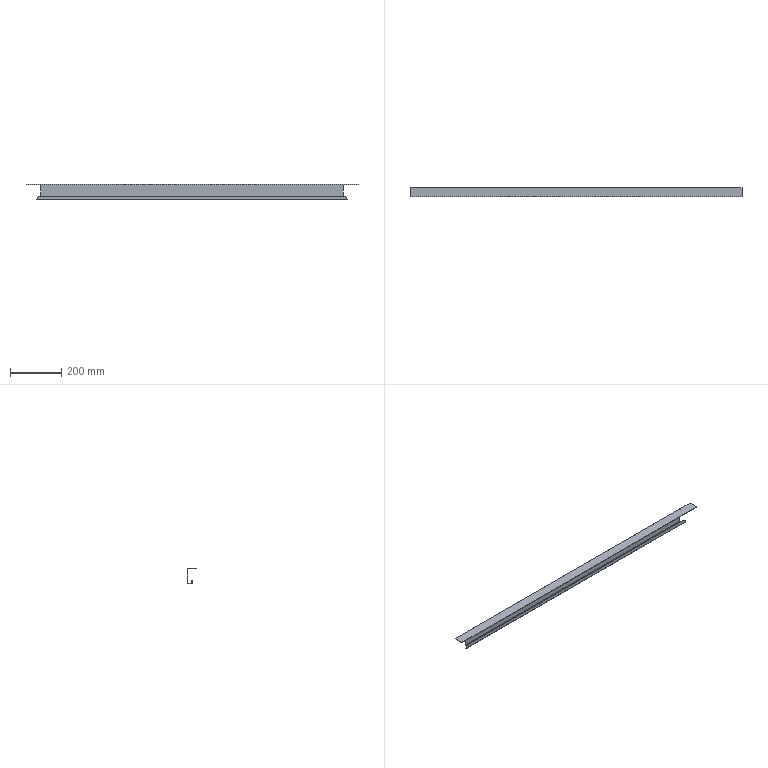Part | SolidWorks | features BaseBody 1 | 1 solid | 44 faces | box 1300 x 39 x 62 mm | volume 312917 mm3 | plane 32 | cylinder 8 | torus 4 | commonest cylinder face diameters 1 x3 5 x3 30 x2
STEP:
#1=CARTESIAN_POINT('',(595.5,0.5,-62.));
#2=VERTEX_POINT('',#1);
#3=CARTESIAN_POINT('',(593.,3.,-62.));
#4=VERTEX_POINT('',#3);
#5=CARTESIAN_POINT('',(595.5,3.,-62.));
#6=DIRECTION('',(0.,0.,-1.));
#7=DIRECTION('',(1.,0.,0.));
#8=AXIS2_PLACEMENT_3D('',#5,#6,#7);
#9=CIRCLE('',#8,2.5);
#10=EDGE_CURVE('',#2,#4,#9,.T.);
#11=ORIENTED_EDGE('',*,*,#10,.T.);
#12=CARTESIAN_POINT('',(595.,3.,-62.));
#13=VERTEX_POINT('',#12);
#14=CARTESIAN_POINT('',(595.,3.,-62.));
#15=DIRECTION('',(1.,0.,0.));
#16=VECTOR('',#15,1000.);
#17=LINE('',#14,#16);
#18=EDGE_CURVE('',#4,#13,#17,.T.);
#19=ORIENTED_EDGE('',*,*,#18,.T.);
#20=CARTESIAN_POINT('',(595.5,2.5,-62.));
#21=VERTEX_POINT('',#20);
#22=CARTESIAN_POINT('',(595.5,3.,-62.));
#23=DIRECTION('',(0.,0.,1.));
#24=DIRECTION('',(1.,0.,0.));
#25=AXIS2_PLACEMENT_3D('',#22,#23,#24);
#26=CIRCLE('',#25,0.5);
#27=EDGE_CURVE('',#13,#21,#26,.T.);
#28=ORIENTED_EDGE('',*,*,#27,.T.);
#29=CARTESIAN_POINT('',(608.,2.5,-62.));
#30=VERTEX_POINT('',#29);
#31=CARTESIAN_POINT('',(608.,2.5,-62.));
#32=DIRECTION('',(1.,0.,0.));
#33=VECTOR('',#32,1000.);
#34=LINE('',#31,#33);
#35=EDGE_CURVE('',#21,#30,#34,.T.);
#36=ORIENTED_EDGE('',*,*,#35,.T.);
#37=CARTESIAN_POINT('',(608.,0.5,-62.));
#38=VERTEX_POINT('',#37);
#39=CARTESIAN_POINT('',(608.,0.5,-62.));
#40=DIRECTION('',(0.,-1.,0.));
#41=VECTOR('',#40,1000.);
#42=LINE('',#39,#41);
#43=EDGE_CURVE('',#30,#38,#42,.T.);
#44=ORIENTED_EDGE('',*,*,#43,.T.);
#45=CARTESIAN_POINT('',(595.5,0.5,-62.));
#46=DIRECTION('',(-1.,0.,0.));
#47=VECTOR('',#46,1000.);
#48=LINE('',#45,#47);
#49=EDGE_CURVE('',#38,#2,#48,.T.);
#50=ORIENTED_EDGE('',*,*,#49,.T.);
#51=EDGE_LOOP('',(#11,#19,#28,#36,#44,#50));
#52=FACE_OUTER_BOUND('',#51,.T.);
#53=CARTESIAN_POINT('',(595.5,3.,-62.));
#54=DIRECTION('',(0.,0.,-1.));
#55=DIRECTION('',(-1.,0.,0.));
#56=AXIS2_PLACEMENT_3D('',#53,#54,#55);
#57=PLANE('',#56);
#58=ADVANCED_FACE('',(#52),#57,.T.);
#59=CARTESIAN_POINT('',(593.,2.5,-59.5));
#60=VERTEX_POINT('',#59);
#61=CARTESIAN_POINT('',(593.,2.5,-62.));
#62=DIRECTION('',(0.,1.,0.));
#63=DIRECTION('',(0.,0.,1.));
#64=AXIS2_PLACEMENT_3D('',#61,#62,#63);
#65=CIRCLE('',#64,2.5);
#66=EDGE_CURVE('',#60,#21,#65,.T.);
#67=ORIENTED_EDGE('',*,*,#66,.T.);
#68=ORIENTED_EDGE('',*,*,#27,.F.);
#69=CARTESIAN_POINT('',(593.,3.,-60.));
#70=VERTEX_POINT('',#69);
#71=CARTESIAN_POINT('',(593.,3.,-62.));
#72=DIRECTION('',(0.,1.,0.));
#73=DIRECTION('',(0.,0.,1.));
#74=AXIS2_PLACEMENT_3D('',#71,#72,#73);
#75=CIRCLE('',#74,2.);
#76=EDGE_CURVE('',#70,#13,#75,.T.);
#77=ORIENTED_EDGE('',*,*,#76,.F.);
#78=CARTESIAN_POINT('',(593.,3.,-59.5));
#79=DIRECTION('',(1.,0.,0.));
#80=DIRECTION('',(0.,0.,-1.));
#81=AXIS2_PLACEMENT_3D('',#78,#79,#80);
#82=CIRCLE('',#81,0.5);
#83=EDGE_CURVE('',#60,#70,#82,.T.);
#84=ORIENTED_EDGE('',*,*,#83,.F.);
#85=EDGE_LOOP('',(#67,#68,#77,#84));
#86=FACE_OUTER_BOUND('',#85,.T.);
#87=CARTESIAN_POINT('',(593.,3.,-62.));
#88=DIRECTION('',(0.,1.,0.));
#89=DIRECTION('',(0.,0.,1.));
#90=AXIS2_PLACEMENT_3D('',#87,#88,#89);
#91=TOROIDAL_SURFACE('',#90,2.5,0.5);
#92=ADVANCED_FACE('',(#86),#91,.F.);
#93=CARTESIAN_POINT('',(593.,0.5,-47.));
#94=VERTEX_POINT('',#93);
#95=CARTESIAN_POINT('',(593.,0.5,-62.));
#96=DIRECTION('',(0.,1.,0.));
#97=DIRECTION('',(0.,0.,1.));
#98=AXIS2_PLACEMENT_3D('',#95,#96,#97);
#99=CIRCLE('',#98,15.);
#100=EDGE_CURVE('',#94,#38,#99,.T.);
#101=ORIENTED_EDGE('',*,*,#100,.T.);
#102=ORIENTED_EDGE('',*,*,#43,.F.);
#103=CARTESIAN_POINT('',(593.,2.5,-47.));
#104=VERTEX_POINT('',#103);
#105=CARTESIAN_POINT('',(593.,2.5,-62.));
#106=DIRECTION('',(0.,1.,0.));
#107=DIRECTION('',(0.,0.,1.));
#108=AXIS2_PLACEMENT_3D('',#105,#106,#107);
#109=CIRCLE('',#108,15.);
#110=EDGE_CURVE('',#104,#30,#109,.T.);
#111=ORIENTED_EDGE('',*,*,#110,.F.);
#112=CARTESIAN_POINT('',(593.,0.5,-47.));
#113=DIRECTION('',(0.,1.,0.));
#114=VECTOR('',#113,1000.);
#115=LINE('',#112,#114);
#116=EDGE_CURVE('',#94,#104,#115,.T.);
#117=ORIENTED_EDGE('',*,*,#116,.F.);
#118=EDGE_LOOP('',(#101,#102,#111,#117));
#119=FACE_OUTER_BOUND('',#118,.T.);
#120=CARTESIAN_POINT('',(593.,0.5,-62.));
#121=DIRECTION('',(0.,1.,0.));
#122=DIRECTION('',(0.,0.,1.));
#123=AXIS2_PLACEMENT_3D('',#120,#121,#122);
#124=CYLINDRICAL_SURFACE('',#123,15.);
#125=ADVANCED_FACE('',(#119),#124,.T.);
#126=CARTESIAN_POINT('',(593.,0.5,-59.5));
#127=VERTEX_POINT('',#126);
#128=CARTESIAN_POINT('',(593.,3.,-59.5));
#129=DIRECTION('',(1.,0.,0.));
#130=DIRECTION('',(0.,0.,-1.));
#131=AXIS2_PLACEMENT_3D('',#128,#129,#130);
#132=CIRCLE('',#131,2.5);
#133=EDGE_CURVE('',#127,#4,#132,.T.);
#134=ORIENTED_EDGE('',*,*,#133,.T.);
#135=ORIENTED_EDGE('',*,*,#10,.F.);
#136=CARTESIAN_POINT('',(593.,0.5,-62.));
#137=DIRECTION('',(0.,1.,0.));
#138=DIRECTION('',(0.,0.,1.));
#139=AXIS2_PLACEMENT_3D('',#136,#137,#138);
#140=CIRCLE('',#139,2.5);
#141=EDGE_CURVE('',#127,#2,#140,.T.);
#142=ORIENTED_EDGE('',*,*,#141,.F.);
#143=EDGE_LOOP('',(#134,#135,#142));
#144=FACE_OUTER_BOUND('',#143,.T.);
#145=CARTESIAN_POINT('',(593.,3.,-62.));
#146=DIRECTION('',(0.,1.,0.));
#147=DIRECTION('',(0.,0.,1.));
#148=AXIS2_PLACEMENT_3D('',#145,#146,#147);
#149=TOROIDAL_SURFACE('',#148,2.5,2.5);
#150=ADVANCED_FACE('',(#144),#149,.T.);
#151=ORIENTED_EDGE('',*,*,#18,.F.);
#152=CARTESIAN_POINT('',(593.,3.,-60.));
#153=DIRECTION('',(0.,0.,-1.));
#154=VECTOR('',#153,1000.);
#155=LINE('',#152,#154);
#156=EDGE_CURVE('',#70,#4,#155,.T.);
#157=ORIENTED_EDGE('',*,*,#156,.F.);
#158=ORIENTED_EDGE('',*,*,#76,.T.);
#159=EDGE_LOOP('',(#151,#157,#158));
#160=FACE_OUTER_BOUND('',#159,.T.);
#161=CARTESIAN_POINT('',(593.,3.,-60.));
#162=DIRECTION('',(0.,1.,0.));
#163=DIRECTION('',(0.,0.,-1.));
#164=AXIS2_PLACEMENT_3D('',#161,#162,#163);
#165=PLANE('',#164);
#166=ADVANCED_FACE('',(#160),#165,.T.);
#167=CARTESIAN_POINT('',(-593.,3.,-62.));
#168=VERTEX_POINT('',#167);
#169=CARTESIAN_POINT('',(-595.5,0.5,-62.));
#170=VERTEX_POINT('',#169);
#171=CARTESIAN_POINT('',(-595.5,3.,-62.));
#172=DIRECTION('',(0.,0.,-1.));
#173=DIRECTION('',(-1.,0.,0.));
#174=AXIS2_PLACEMENT_3D('',#171,#172,#173);
#175=CIRCLE('',#174,2.5);
#176=EDGE_CURVE('',#168,#170,#175,.T.);
#177=ORIENTED_EDGE('',*,*,#176,.T.);
#178=CARTESIAN_POINT('',(-608.,0.5,-62.));
#179=VERTEX_POINT('',#178);
#180=CARTESIAN_POINT('',(-595.5,0.5,-62.));
#181=DIRECTION('',(-1.,0.,0.));
#182=VECTOR('',#181,1000.);
#183=LINE('',#180,#182);
#184=EDGE_CURVE('',#170,#179,#183,.T.);
#185=ORIENTED_EDGE('',*,*,#184,.T.);
#186=CARTESIAN_POINT('',(-608.,2.5,-62.));
#187=VERTEX_POINT('',#186);
#188=CARTESIAN_POINT('',(-608.,0.5,-62.));
#189=DIRECTION('',(0.,1.,0.));
#190=VECTOR('',#189,1000.);
#191=LINE('',#188,#190);
#192=EDGE_CURVE('',#179,#187,#191,.T.);
#193=ORIENTED_EDGE('',*,*,#192,.T.);
#194=CARTESIAN_POINT('',(-595.5,2.5,-62.));
#195=VERTEX_POINT('',#194);
#196=CARTESIAN_POINT('',(-608.,2.5,-62.));
#197=DIRECTION('',(1.,0.,0.));
#198=VECTOR('',#197,1000.);
#199=LINE('',#196,#198);
#200=EDGE_CURVE('',#187,#195,#199,.T.);
#201=ORIENTED_EDGE('',*,*,#200,.T.);
#202=CARTESIAN_POINT('',(-595.,3.,-62.));
#203=VERTEX_POINT('',#202);
#204=CARTESIAN_POINT('',(-595.5,3.,-62.));
#205=DIRECTION('',(0.,0.,1.));
#206=DIRECTION('',(-1.,0.,0.));
#207=AXIS2_PLACEMENT_3D('',#204,#205,#206);
#208=CIRCLE('',#207,0.5);
#209=EDGE_CURVE('',#195,#203,#208,.T.);
#210=ORIENTED_EDGE('',*,*,#209,.T.);
#211=CARTESIAN_POINT('',(-595.,3.,-62.));
#212=DIRECTION('',(1.,0.,0.));
#213=VECTOR('',#212,1000.);
#214=LINE('',#211,#213);
#215=EDGE_CURVE('',#203,#168,#214,.T.);
#216=ORIENTED_EDGE('',*,*,#215,.T.);
#217=EDGE_LOOP('',(#177,#185,#193,#201,#210,#216));
#218=FACE_OUTER_BOUND('',#217,.T.);
#219=CARTESIAN_POINT('',(-595.5,3.,-62.));
#220=DIRECTION('',(0.,0.,-1.));
#221=DIRECTION('',(-1.,0.,0.));
#222=AXIS2_PLACEMENT_3D('',#219,#220,#221);
#223=PLANE('',#222);
#224=ADVANCED_FACE('',(#218),#223,.T.);
#225=CARTESIAN_POINT('',(-593.,0.5,-59.5));
#226=VERTEX_POINT('',#225);
#227=CARTESIAN_POINT('',(-593.,0.5,-62.));
#228=DIRECTION('',(0.,-1.,0.));
#229=DIRECTION('',(0.,0.,1.));
#230=AXIS2_PLACEMENT_3D('',#227,#228,#229);
#231=CIRCLE('',#230,2.5);
#232=EDGE_CURVE('',#226,#170,#231,.T.);
#233=ORIENTED_EDGE('',*,*,#232,.T.);
#234=ORIENTED_EDGE('',*,*,#176,.F.);
#235=CARTESIAN_POINT('',(-593.,3.,-59.5));
#236=DIRECTION('',(-1.,0.,0.));
#237=DIRECTION('',(0.,0.,-1.));
#238=AXIS2_PLACEMENT_3D('',#235,#236,#237);
#239=CIRCLE('',#238,2.5);
#240=EDGE_CURVE('',#168,#226,#239,.T.);
#241=ORIENTED_EDGE('',*,*,#240,.T.);
#242=EDGE_LOOP('',(#233,#234,#241));
#243=FACE_OUTER_BOUND('',#242,.T.);
#244=CARTESIAN_POINT('',(-593.,3.,-62.));
#245=DIRECTION('',(0.,-1.,0.));
#246=DIRECTION('',(0.,0.,-1.));
#247=AXIS2_PLACEMENT_3D('',#244,#245,#246);
#248=TOROIDAL_SURFACE('',#247,2.5,2.5);
#249=ADVANCED_FACE('',(#243),#248,.T.);
#250=CARTESIAN_POINT('',(-593.,2.5,-47.));
#251=VERTEX_POINT('',#250);
#252=CARTESIAN_POINT('',(-593.,2.5,-62.));
#253=DIRECTION('',(0.,-1.,0.));
#254=DIRECTION('',(0.,0.,1.));
#255=AXIS2_PLACEMENT_3D('',#252,#253,#254);
#256=CIRCLE('',#255,15.);
#257=EDGE_CURVE('',#251,#187,#256,.T.);
#258=ORIENTED_EDGE('',*,*,#257,.T.);
#259=ORIENTED_EDGE('',*,*,#192,.F.);
#260=CARTESIAN_POINT('',(-593.,0.5,-47.));
#261=VERTEX_POINT('',#260);
#262=CARTESIAN_POINT('',(-593.,0.5,-62.));
#263=DIRECTION('',(0.,-1.,0.));
#264=DIRECTION('',(0.,0.,1.));
#265=AXIS2_PLACEMENT_3D('',#262,#263,#264);
#266=CIRCLE('',#265,15.);
#267=EDGE_CURVE('',#261,#179,#266,.T.);
#268=ORIENTED_EDGE('',*,*,#267,.F.);
#269=CARTESIAN_POINT('',(-593.,0.5,-47.));
#270=DIRECTION('',(0.,1.,0.));
#271=VECTOR('',#270,1000.);
#272=LINE('',#269,#271);
#273=EDGE_CURVE('',#261,#251,#272,.T.);
#274=ORIENTED_EDGE('',*,*,#273,.T.);
#275=EDGE_LOOP('',(#258,#259,#268,#274));
#276=FACE_OUTER_BOUND('',#275,.T.);
#277=CARTESIAN_POINT('',(-593.,0.5,-62.));
#278=DIRECTION('',(0.,-1.,0.));
#279=DIRECTION('',(0.,0.,-1.));
#280=AXIS2_PLACEMENT_3D('',#277,#278,#279);
#281=CYLINDRICAL_SURFACE('',#280,15.);
#282=ADVANCED_FACE('',(#276),#281,.T.);
#283=CARTESIAN_POINT('',(-593.,3.,-60.));
#284=VERTEX_POINT('',#283);
#285=CARTESIAN_POINT('',(-593.,3.,-62.));
#286=DIRECTION('',(0.,-1.,0.));
#287=DIRECTION('',(0.,0.,1.));
#288=AXIS2_PLACEMENT_3D('',#285,#286,#287);
#289=CIRCLE('',#288,2.);
#290=EDGE_CURVE('',#284,#203,#289,.T.);
#291=ORIENTED_EDGE('',*,*,#290,.T.);
#292=ORIENTED_EDGE('',*,*,#209,.F.);
#293=CARTESIAN_POINT('',(-593.,2.5,-59.5));
#294=VERTEX_POINT('',#293);
#295=CARTESIAN_POINT('',(-593.,2.5,-62.));
#296=DIRECTION('',(0.,-1.,0.));
#297=DIRECTION('',(0.,0.,1.));
#298=AXIS2_PLACEMENT_3D('',#295,#296,#297);
#299=CIRCLE('',#298,2.5);
#300=EDGE_CURVE('',#294,#195,#299,.T.);
#301=ORIENTED_EDGE('',*,*,#300,.F.);
#302=CARTESIAN_POINT('',(-593.,3.,-59.5));
#303=DIRECTION('',(-1.,0.,0.));
#304=DIRECTION('',(0.,0.,-1.));
#305=AXIS2_PLACEMENT_3D('',#302,#303,#304);
#306=CIRCLE('',#305,0.5);
#307=EDGE_CURVE('',#284,#294,#306,.T.);
#308=ORIENTED_EDGE('',*,*,#307,.F.);
#309=EDGE_LOOP('',(#291,#292,#301,#308));
#310=FACE_OUTER_BOUND('',#309,.T.);
#311=CARTESIAN_POINT('',(-593.,3.,-62.));
#312=DIRECTION('',(0.,-1.,0.));
#313=DIRECTION('',(0.,0.,-1.));
#314=AXIS2_PLACEMENT_3D('',#311,#312,#313);
#315=TOROIDAL_SURFACE('',#314,2.5,0.5);
#316=ADVANCED_FACE('',(#310),#315,.F.);
#317=ORIENTED_EDGE('',*,*,#215,.F.);
#318=ORIENTED_EDGE('',*,*,#290,.F.);
#319=CARTESIAN_POINT('',(-593.,3.,-60.));
#320=DIRECTION('',(0.,0.,-1.));
#321=VECTOR('',#320,1000.);
#322=LINE('',#319,#321);
#323=EDGE_CURVE('',#284,#168,#322,.T.);
#324=ORIENTED_EDGE('',*,*,#323,.T.);
#325=EDGE_LOOP('',(#317,#318,#324));
#326=FACE_OUTER_BOUND('',#325,.T.);
#327=CARTESIAN_POINT('',(-593.,3.,-60.));
#328=DIRECTION('',(0.,1.,0.));
#329=DIRECTION('',(0.,0.,-1.));
#330=AXIS2_PLACEMENT_3D('',#327,#328,#329);
#331=PLANE('',#330);
#332=ADVANCED_FACE('',(#326),#331,.T.);
#333=CARTESIAN_POINT('',(-593.,2.5,-47.));
#334=DIRECTION('',(-1.,0.,0.));
#335=VECTOR('',#334,1000.);
#336=LINE('',#333,#335);
#337=EDGE_CURVE('',#104,#251,#336,.T.);
#338=ORIENTED_EDGE('',*,*,#337,.T.);
#339=ORIENTED_EDGE('',*,*,#273,.F.);
#340=CARTESIAN_POINT('',(0.,0.5,-47.));
#341=DIRECTION('',(-1.,0.,0.));
#342=VECTOR('',#341,1000.);
#343=LINE('',#340,#342);
#344=EDGE_CURVE('',#94,#261,#343,.T.);
#345=ORIENTED_EDGE('',*,*,#344,.F.);
#346=ORIENTED_EDGE('',*,*,#116,.T.);
#347=EDGE_LOOP('',(#338,#339,#345,#346));
#348=FACE_OUTER_BOUND('',#347,.T.);
#349=CARTESIAN_POINT('',(-593.,0.5,-47.));
#350=DIRECTION('',(0.,0.,-1.));
#351=DIRECTION('',(-1.,0.,0.));
#352=AXIS2_PLACEMENT_3D('',#349,#350,#351);
#353=PLANE('',#352);
#354=ADVANCED_FACE('',(#348),#353,.F.);
#355=ORIENTED_EDGE('',*,*,#337,.F.);
#356=ORIENTED_EDGE('',*,*,#110,.T.);
#357=ORIENTED_EDGE('',*,*,#35,.F.);
#358=ORIENTED_EDGE('',*,*,#66,.F.);
#359=CARTESIAN_POINT('',(-593.,2.5,-59.5));
#360=DIRECTION('',(1.,0.,0.));
#361=VECTOR('',#360,1000.);
#362=LINE('',#359,#361);
#363=EDGE_CURVE('',#294,#60,#362,.T.);
#364=ORIENTED_EDGE('',*,*,#363,.F.);
#365=ORIENTED_EDGE('',*,*,#300,.T.);
#366=ORIENTED_EDGE('',*,*,#200,.F.);
#367=ORIENTED_EDGE('',*,*,#257,.F.);
#368=EDGE_LOOP('',(#355,#356,#357,#358,#364,#365,#366,#367));
#369=FACE_OUTER_BOUND('',#368,.T.);
#370=CARTESIAN_POINT('',(0.,2.5,0.));
#371=DIRECTION('',(0.,1.,0.));
#372=DIRECTION('',(0.,0.,-1.));
#373=AXIS2_PLACEMENT_3D('',#370,#371,#372);
#374=PLANE('',#373);
#375=ADVANCED_FACE('',(#369),#374,.T.);
#376=CARTESIAN_POINT('',(-593.,0.5,-59.5));
#377=DIRECTION('',(-1.,0.,0.));
#378=VECTOR('',#377,1000.);
#379=LINE('',#376,#378);
#380=EDGE_CURVE('',#127,#226,#379,.T.);
#381=ORIENTED_EDGE('',*,*,#380,.F.);
#382=ORIENTED_EDGE('',*,*,#141,.T.);
#383=ORIENTED_EDGE('',*,*,#49,.F.);
#384=ORIENTED_EDGE('',*,*,#100,.F.);
#385=ORIENTED_EDGE('',*,*,#344,.T.);
#386=ORIENTED_EDGE('',*,*,#267,.T.);
#387=ORIENTED_EDGE('',*,*,#184,.F.);
#388=ORIENTED_EDGE('',*,*,#232,.F.);
#389=EDGE_LOOP('',(#381,#382,#383,#384,#385,#386,#387,#388));
#390=FACE_OUTER_BOUND('',#389,.T.);
#391=CARTESIAN_POINT('',(0.,0.5,0.));
#392=DIRECTION('',(0.,1.,0.));
#393=DIRECTION('',(0.,0.,-1.));
#394=AXIS2_PLACEMENT_3D('',#391,#392,#393);
#395=PLANE('',#394);
#396=ADVANCED_FACE('',(#390),#395,.F.);
#397=CARTESIAN_POINT('',(593.,3.,-60.));
#398=DIRECTION('',(-1.,0.,0.));
#399=VECTOR('',#398,1000.);
#400=LINE('',#397,#399);
#401=EDGE_CURVE('',#70,#284,#400,.T.);
#402=ORIENTED_EDGE('',*,*,#401,.T.);
#403=ORIENTED_EDGE('',*,*,#307,.T.);
#404=ORIENTED_EDGE('',*,*,#363,.T.);
#405=ORIENTED_EDGE('',*,*,#83,.T.);
#406=EDGE_LOOP('',(#402,#403,#404,#405));
#407=FACE_OUTER_BOUND('',#406,.T.);
#408=CARTESIAN_POINT('',(593.,3.,-59.5));
#409=DIRECTION('',(1.,0.,0.));
#410=DIRECTION('',(0.,-1.,0.));
#411=AXIS2_PLACEMENT_3D('',#408,#409,#410);
#412=CYLINDRICAL_SURFACE('',#411,0.5);
#413=ADVANCED_FACE('',(#407),#412,.F.);
#414=CARTESIAN_POINT('',(593.,3.,-62.));
#415=DIRECTION('',(-1.,0.,0.));
#416=VECTOR('',#415,1000.);
#417=LINE('',#414,#416);
#418=EDGE_CURVE('',#4,#168,#417,.T.);
#419=ORIENTED_EDGE('',*,*,#418,.F.);
#420=ORIENTED_EDGE('',*,*,#133,.F.);
#421=ORIENTED_EDGE('',*,*,#380,.T.);
#422=ORIENTED_EDGE('',*,*,#240,.F.);
#423=EDGE_LOOP('',(#419,#420,#421,#422));
#424=FACE_OUTER_BOUND('',#423,.T.);
#425=CARTESIAN_POINT('',(593.,3.,-59.5));
#426=DIRECTION('',(1.,0.,0.));
#427=DIRECTION('',(0.,-1.,0.));
#428=AXIS2_PLACEMENT_3D('',#425,#426,#427);
#429=CYLINDRICAL_SURFACE('',#428,2.5);
#430=ADVANCED_FACE('',(#424),#429,.T.);
#431=CARTESIAN_POINT('',(593.,18.5,-59.5));
#432=VERTEX_POINT('',#431);
#433=CARTESIAN_POINT('',(-593.,18.5,-59.5));
#434=VERTEX_POINT('',#433);
#435=CARTESIAN_POINT('',(593.,18.5,-59.5));
#436=DIRECTION('',(-1.,0.,0.));
#437=VECTOR('',#436,1000.);
#438=LINE('',#435,#437);
#439=EDGE_CURVE('',#432,#434,#438,.T.);
#440=ORIENTED_EDGE('',*,*,#439,.T.);
#441=CARTESIAN_POINT('',(-593.,18.,-60.));
#442=VERTEX_POINT('',#441);
#443=CARTESIAN_POINT('',(-593.,18.,-59.5));
#444=DIRECTION('',(-1.,0.,0.));
#445=DIRECTION('',(0.,0.,-1.));
#446=AXIS2_PLACEMENT_3D('',#443,#444,#445);
#447=CIRCLE('',#446,0.5);
#448=EDGE_CURVE('',#434,#442,#447,.T.);
#449=ORIENTED_EDGE('',*,*,#448,.T.);
#450=CARTESIAN_POINT('',(593.,18.,-60.));
#451=VERTEX_POINT('',#450);
#452=CARTESIAN_POINT('',(-593.,18.,-60.));
#453=DIRECTION('',(1.,0.,0.));
#454=VECTOR('',#453,1000.);
#455=LINE('',#452,#454);
#456=EDGE_CURVE('',#442,#451,#455,.T.);
#457=ORIENTED_EDGE('',*,*,#456,.T.);
#458=CARTESIAN_POINT('',(593.,18.,-59.5));
#459=DIRECTION('',(1.,0.,0.));
#460=DIRECTION('',(0.,0.,-1.));
#461=AXIS2_PLACEMENT_3D('',#458,#459,#460);
#462=CIRCLE('',#461,0.5);
#463=EDGE_CURVE('',#451,#432,#462,.T.);
#464=ORIENTED_EDGE('',*,*,#463,.T.);
#465=EDGE_LOOP('',(#440,#449,#457,#464));
#466=FACE_OUTER_BOUND('',#465,.T.);
#467=CARTESIAN_POINT('',(593.,18.,-59.5));
#468=DIRECTION('',(1.,0.,0.));
#469=DIRECTION('',(0.,0.,-1.));
#470=AXIS2_PLACEMENT_3D('',#467,#468,#469);
#471=CYLINDRICAL_SURFACE('',#470,0.5);
#472=ADVANCED_FACE('',(#466),#471,.F.);
#473=CARTESIAN_POINT('',(593.,20.5,-59.5));
#474=VERTEX_POINT('',#473);
#475=CARTESIAN_POINT('',(-593.,20.5,-59.5));
#476=VERTEX_POINT('',#475);
#477=CARTESIAN_POINT('',(593.,20.5,-59.5));
#478=DIRECTION('',(-1.,0.,0.));
#479=VECTOR('',#478,1000.);
#480=LINE('',#477,#479);
#481=EDGE_CURVE('',#474,#476,#480,.T.);
#482=ORIENTED_EDGE('',*,*,#481,.F.);
#483=CARTESIAN_POINT('',(593.,18.,-62.));
#484=VERTEX_POINT('',#483);
#485=CARTESIAN_POINT('',(593.,18.,-59.5));
#486=DIRECTION('',(1.,0.,0.));
#487=DIRECTION('',(0.,0.,-1.));
#488=AXIS2_PLACEMENT_3D('',#485,#486,#487);
#489=CIRCLE('',#488,2.5);
#490=EDGE_CURVE('',#484,#474,#489,.T.);
#491=ORIENTED_EDGE('',*,*,#490,.F.);
#492=CARTESIAN_POINT('',(-593.,18.,-62.));
#493=VERTEX_POINT('',#492);
#494=CARTESIAN_POINT('',(-593.,18.,-62.));
#495=DIRECTION('',(-1.,0.,0.));
#496=VECTOR('',#495,1000.);
#497=LINE('',#494,#496);
#498=EDGE_CURVE('',#484,#493,#497,.T.);
#499=ORIENTED_EDGE('',*,*,#498,.T.);
#500=CARTESIAN_POINT('',(-593.,18.,-59.5));
#501=DIRECTION('',(-1.,0.,0.));
#502=DIRECTION('',(0.,0.,-1.));
#503=AXIS2_PLACEMENT_3D('',#500,#501,#502);
#504=CIRCLE('',#503,2.5);
#505=EDGE_CURVE('',#476,#493,#504,.T.);
#506=ORIENTED_EDGE('',*,*,#505,.F.);
#507=EDGE_LOOP('',(#482,#491,#499,#506));
#508=FACE_OUTER_BOUND('',#507,.T.);
#509=CARTESIAN_POINT('',(593.,18.,-59.5));
#510=DIRECTION('',(1.,0.,0.));
#511=DIRECTION('',(0.,0.,-1.));
#512=AXIS2_PLACEMENT_3D('',#509,#510,#511);
#513=CYLINDRICAL_SURFACE('',#512,2.5);
#514=ADVANCED_FACE('',(#508),#513,.T.);
#515=ORIENTED_EDGE('',*,*,#463,.F.);
#516=CARTESIAN_POINT('',(593.,18.,-60.));
#517=DIRECTION('',(0.,0.,-1.));
#518=VECTOR('',#517,1000.);
#519=LINE('',#516,#518);
#520=EDGE_CURVE('',#451,#484,#519,.T.);
#521=ORIENTED_EDGE('',*,*,#520,.T.);
#522=ORIENTED_EDGE('',*,*,#490,.T.);
#523=CARTESIAN_POINT('',(593.,18.5,-59.5));
#524=DIRECTION('',(0.,1.,0.));
#525=VECTOR('',#524,1000.);
#526=LINE('',#523,#525);
#527=EDGE_CURVE('',#432,#474,#526,.T.);
#528=ORIENTED_EDGE('',*,*,#527,.F.);
#529=EDGE_LOOP('',(#515,#521,#522,#528));
#530=FACE_OUTER_BOUND('',#529,.T.);
#531=CARTESIAN_POINT('',(593.,18.,-59.5));
#532=DIRECTION('',(-1.,0.,0.));
#533=DIRECTION('',(0.,0.,1.));
#534=AXIS2_PLACEMENT_3D('',#531,#532,#533);
#535=PLANE('',#534);
#536=ADVANCED_FACE('',(#530),#535,.F.);
#537=CARTESIAN_POINT('',(-593.,18.,-62.));
#538=DIRECTION('',(0.,0.,-1.));
#539=VECTOR('',#538,1000.);
#540=LINE('',#537,#539);
#541=EDGE_CURVE('',#442,#493,#540,.T.);
#542=ORIENTED_EDGE('',*,*,#541,.F.);
#543=ORIENTED_EDGE('',*,*,#448,.F.);
#544=CARTESIAN_POINT('',(-593.,18.5,-59.5));
#545=DIRECTION('',(0.,1.,0.));
#546=VECTOR('',#545,1000.);
#547=LINE('',#544,#546);
#548=EDGE_CURVE('',#434,#476,#547,.T.);
#549=ORIENTED_EDGE('',*,*,#548,.T.);
#550=ORIENTED_EDGE('',*,*,#505,.T.);
#551=EDGE_LOOP('',(#542,#543,#549,#550));
#552=FACE_OUTER_BOUND('',#551,.T.);
#553=CARTESIAN_POINT('',(-593.,18.,-59.5));
#554=DIRECTION('',(-1.,0.,0.));
#555=DIRECTION('',(0.,0.,1.));
#556=AXIS2_PLACEMENT_3D('',#553,#554,#555);
#557=PLANE('',#556);
#558=ADVANCED_FACE('',(#552),#557,.T.);
#559=CARTESIAN_POINT('',(593.,18.,-2.));
#560=VERTEX_POINT('',#559);
#561=CARTESIAN_POINT('',(-593.,18.,-2.));
#562=VERTEX_POINT('',#561);
#563=CARTESIAN_POINT('',(593.,18.,-2.));
#564=DIRECTION('',(-1.,0.,0.));
#565=VECTOR('',#564,1000.);
#566=LINE('',#563,#565);
#567=EDGE_CURVE('',#560,#562,#566,.T.);
#568=ORIENTED_EDGE('',*,*,#567,.T.);
#569=CARTESIAN_POINT('',(-593.,18.5,-2.5));
#570=VERTEX_POINT('',#569);
#571=CARTESIAN_POINT('',(-593.,18.,-2.5));
#572=DIRECTION('',(-1.,0.,0.));
#573=DIRECTION('',(0.,0.,-1.));
#574=AXIS2_PLACEMENT_3D('',#571,#572,#573);
#575=CIRCLE('',#574,0.5);
#576=EDGE_CURVE('',#562,#570,#575,.T.);
#577=ORIENTED_EDGE('',*,*,#576,.T.);
#578=CARTESIAN_POINT('',(593.,18.5,-2.5));
#579=VERTEX_POINT('',#578);
#580=CARTESIAN_POINT('',(-593.,18.5,-2.5));
#581=DIRECTION('',(1.,0.,0.));
#582=VECTOR('',#581,1000.);
#583=LINE('',#580,#582);
#584=EDGE_CURVE('',#570,#579,#583,.T.);
#585=ORIENTED_EDGE('',*,*,#584,.T.);
#586=CARTESIAN_POINT('',(593.,18.,-2.5));
#587=DIRECTION('',(1.,0.,0.));
#588=DIRECTION('',(0.,0.,-1.));
#589=AXIS2_PLACEMENT_3D('',#586,#587,#588);
#590=CIRCLE('',#589,0.5);
#591=EDGE_CURVE('',#579,#560,#590,.T.);
#592=ORIENTED_EDGE('',*,*,#591,.T.);
#593=EDGE_LOOP('',(#568,#577,#585,#592));
#594=FACE_OUTER_BOUND('',#593,.T.);
#595=CARTESIAN_POINT('',(593.,18.,-2.5));
#596=DIRECTION('',(1.,0.,0.));
#597=DIRECTION('',(0.,1.,0.));
#598=AXIS2_PLACEMENT_3D('',#595,#596,#597);
#599=CYLINDRICAL_SURFACE('',#598,0.5);
#600=ADVANCED_FACE('',(#594),#599,.F.);
#601=CARTESIAN_POINT('',(593.,18.,0.));
#602=VERTEX_POINT('',#601);
#603=CARTESIAN_POINT('',(-593.,18.,0.));
#604=VERTEX_POINT('',#603);
#605=CARTESIAN_POINT('',(593.,18.,0.));
#606=DIRECTION('',(-1.,0.,0.));
#607=VECTOR('',#606,1000.);
#608=LINE('',#605,#607);
#609=EDGE_CURVE('',#602,#604,#608,.T.);
#610=ORIENTED_EDGE('',*,*,#609,.F.);
#611=CARTESIAN_POINT('',(593.,20.5,-2.5));
#612=VERTEX_POINT('',#611);
#613=CARTESIAN_POINT('',(593.,18.,-2.5));
#614=DIRECTION('',(1.,0.,0.));
#615=DIRECTION('',(0.,0.,-1.));
#616=AXIS2_PLACEMENT_3D('',#613,#614,#615);
#617=CIRCLE('',#616,2.5);
#618=EDGE_CURVE('',#612,#602,#617,.T.);
#619=ORIENTED_EDGE('',*,*,#618,.F.);
#620=CARTESIAN_POINT('',(-593.,20.5,-2.5));
#621=VERTEX_POINT('',#620);
#622=CARTESIAN_POINT('',(0.,20.5,-2.5));
#623=DIRECTION('',(-1.,0.,0.));
#624=VECTOR('',#623,1000.);
#625=LINE('',#622,#624);
#626=EDGE_CURVE('',#612,#621,#625,.T.);
#627=ORIENTED_EDGE('',*,*,#626,.T.);
#628=CARTESIAN_POINT('',(-593.,18.,-2.5));
#629=DIRECTION('',(-1.,0.,0.));
#630=DIRECTION('',(0.,0.,-1.));
#631=AXIS2_PLACEMENT_3D('',#628,#629,#630);
#632=CIRCLE('',#631,2.5);
#633=EDGE_CURVE('',#604,#621,#632,.T.);
#634=ORIENTED_EDGE('',*,*,#633,.F.);
#635=EDGE_LOOP('',(#610,#619,#627,#634));
#636=FACE_OUTER_BOUND('',#635,.T.);
#637=CARTESIAN_POINT('',(593.,18.,-2.5));
#638=DIRECTION('',(1.,0.,0.));
#639=DIRECTION('',(0.,1.,0.));
#640=AXIS2_PLACEMENT_3D('',#637,#638,#639);
#641=CYLINDRICAL_SURFACE('',#640,2.5);
#642=ADVANCED_FACE('',(#636),#641,.T.);
#643=ORIENTED_EDGE('',*,*,#591,.F.);
#644=CARTESIAN_POINT('',(593.,18.5,-2.5));
#645=DIRECTION('',(0.,1.,0.));
#646=VECTOR('',#645,1000.);
#647=LINE('',#644,#646);
#648=EDGE_CURVE('',#579,#612,#647,.T.);
#649=ORIENTED_EDGE('',*,*,#648,.T.);
#650=ORIENTED_EDGE('',*,*,#618,.T.);
#651=CARTESIAN_POINT('',(593.,18.,-2.));
#652=DIRECTION('',(0.,0.,1.));
#653=VECTOR('',#652,1000.);
#654=LINE('',#651,#653);
#655=EDGE_CURVE('',#560,#602,#654,.T.);
#656=ORIENTED_EDGE('',*,*,#655,.F.);
#657=EDGE_LOOP('',(#643,#649,#650,#656));
#658=FACE_OUTER_BOUND('',#657,.T.);
#659=CARTESIAN_POINT('',(593.,18.,-2.5));
#660=DIRECTION('',(-1.,0.,0.));
#661=DIRECTION('',(0.,0.,1.));
#662=AXIS2_PLACEMENT_3D('',#659,#660,#661);
#663=PLANE('',#662);
#664=ADVANCED_FACE('',(#658),#663,.F.);
#665=CARTESIAN_POINT('',(-593.,18.5,-2.5));
#666=DIRECTION('',(0.,1.,0.));
#667=VECTOR('',#666,1000.);
#668=LINE('',#665,#667);
#669=EDGE_CURVE('',#570,#621,#668,.T.);
#670=ORIENTED_EDGE('',*,*,#669,.F.);
#671=ORIENTED_EDGE('',*,*,#576,.F.);
#672=CARTESIAN_POINT('',(-593.,18.,-2.));
#673=DIRECTION('',(0.,0.,1.));
#674=VECTOR('',#673,1000.);
#675=LINE('',#672,#674);
#676=EDGE_CURVE('',#562,#604,#675,.T.);
#677=ORIENTED_EDGE('',*,*,#676,.T.);
#678=ORIENTED_EDGE('',*,*,#633,.T.);
#679=EDGE_LOOP('',(#670,#671,#677,#678));
#680=FACE_OUTER_BOUND('',#679,.T.);
#681=CARTESIAN_POINT('',(-593.,18.,-2.5));
#682=DIRECTION('',(-1.,0.,0.));
#683=DIRECTION('',(0.,0.,1.));
#684=AXIS2_PLACEMENT_3D('',#681,#682,#683);
#685=PLANE('',#684);
#686=ADVANCED_FACE('',(#680),#685,.T.);
#687=CARTESIAN_POINT('',(-594.,18.5,-2.));
#688=VERTEX_POINT('',#687);
#689=CARTESIAN_POINT('',(-594.,18.5,0.));
#690=VERTEX_POINT('',#689);
#691=CARTESIAN_POINT('',(-594.,18.5,-2.));
#692=DIRECTION('',(0.,0.,1.));
#693=VECTOR('',#692,1000.);
#694=LINE('',#691,#693);
#695=EDGE_CURVE('',#688,#690,#694,.T.);
#696=ORIENTED_EDGE('',*,*,#695,.T.);
#697=CARTESIAN_POINT('',(-594.,17.,0.));
#698=VERTEX_POINT('',#697);
#699=CARTESIAN_POINT('',(-594.,0.,0.));
#700=DIRECTION('',(0.,-1.,0.));
#701=VECTOR('',#700,1000.);
#702=LINE('',#699,#701);
#703=EDGE_CURVE('',#690,#698,#702,.T.);
#704=ORIENTED_EDGE('',*,*,#703,.T.);
#705=CARTESIAN_POINT('',(-594.,17.,-2.));
#706=VERTEX_POINT('',#705);
#707=CARTESIAN_POINT('',(-594.,17.,-2.));
#708=DIRECTION('',(0.,0.,1.));
#709=VECTOR('',#708,1000.);
#710=LINE('',#707,#709);
#711=EDGE_CURVE('',#706,#698,#710,.T.);
#712=ORIENTED_EDGE('',*,*,#711,.F.);
#713=CARTESIAN_POINT('',(-594.,17.,-2.));
#714=DIRECTION('',(0.,1.,0.));
#715=VECTOR('',#714,1000.);
#716=LINE('',#713,#715);
#717=EDGE_CURVE('',#706,#688,#716,.T.);
#718=ORIENTED_EDGE('',*,*,#717,.T.);
#719=EDGE_LOOP('',(#696,#704,#712,#718));
#720=FACE_OUTER_BOUND('',#719,.T.);
#721=CARTESIAN_POINT('',(-594.,17.,-2.));
#722=DIRECTION('',(1.,0.,0.));
#723=DIRECTION('',(0.,1.,0.));
#724=AXIS2_PLACEMENT_3D('',#721,#722,#723);
#725=PLANE('',#724);
#726=ADVANCED_FACE('',(#720),#725,.T.);
#727=ORIENTED_EDGE('',*,*,#711,.T.);
#728=CARTESIAN_POINT('',(-593.,17.,0.));
#729=VERTEX_POINT('',#728);
#730=CARTESIAN_POINT('',(0.,17.,0.));
#731=DIRECTION('',(1.,0.,0.));
#732=VECTOR('',#731,1000.);
#733=LINE('',#730,#732);
#734=EDGE_CURVE('',#698,#729,#733,.T.);
#735=ORIENTED_EDGE('',*,*,#734,.T.);
#736=CARTESIAN_POINT('',(-593.,17.,-2.));
#737=VERTEX_POINT('',#736);
#738=CARTESIAN_POINT('',(-593.,17.,-2.));
#739=DIRECTION('',(0.,0.,1.));
#740=VECTOR('',#739,1000.);
#741=LINE('',#738,#740);
#742=EDGE_CURVE('',#737,#729,#741,.T.);
#743=ORIENTED_EDGE('',*,*,#742,.F.);
#744=CARTESIAN_POINT('',(-593.,17.,-2.));
#745=DIRECTION('',(-1.,0.,0.));
#746=VECTOR('',#745,1000.);
#747=LINE('',#744,#746);
#748=EDGE_CURVE('',#737,#706,#747,.T.);
#749=ORIENTED_EDGE('',*,*,#748,.T.);
#750=EDGE_LOOP('',(#727,#735,#743,#749));
#751=FACE_OUTER_BOUND('',#750,.T.);
#752=CARTESIAN_POINT('',(-593.,17.,-2.));
#753=DIRECTION('',(0.,1.,0.));
#754=DIRECTION('',(1.,0.,0.));
#755=AXIS2_PLACEMENT_3D('',#752,#753,#754);
#756=PLANE('',#755);
#757=ADVANCED_FACE('',(#751),#756,.T.);
#758=ORIENTED_EDGE('',*,*,#742,.T.);
#759=CARTESIAN_POINT('',(-593.,0.,0.));
#760=DIRECTION('',(0.,1.,0.));
#761=VECTOR('',#760,1000.);
#762=LINE('',#759,#761);
#763=EDGE_CURVE('',#729,#604,#762,.T.);
#764=ORIENTED_EDGE('',*,*,#763,.T.);
#765=ORIENTED_EDGE('',*,*,#676,.F.);
#766=CARTESIAN_POINT('',(-593.,18.,-2.));
#767=DIRECTION('',(0.,-1.,0.));
#768=VECTOR('',#767,1000.);
#769=LINE('',#766,#768);
#770=EDGE_CURVE('',#562,#737,#769,.T.);
#771=ORIENTED_EDGE('',*,*,#770,.T.);
#772=EDGE_LOOP('',(#758,#764,#765,#771));
#773=FACE_OUTER_BOUND('',#772,.T.);
#774=CARTESIAN_POINT('',(-593.,18.,-2.));
#775=DIRECTION('',(-1.,0.,0.));
#776=DIRECTION('',(0.,0.,1.));
#777=AXIS2_PLACEMENT_3D('',#774,#775,#776);
#778=PLANE('',#777);
#779=ADVANCED_FACE('',(#773),#778,.T.);
#780=ORIENTED_EDGE('',*,*,#655,.T.);
#781=CARTESIAN_POINT('',(593.,17.,0.));
#782=VERTEX_POINT('',#781);
#783=CARTESIAN_POINT('',(593.,0.,0.));
#784=DIRECTION('',(0.,-1.,0.));
#785=VECTOR('',#784,1000.);
#786=LINE('',#783,#785);
#787=EDGE_CURVE('',#602,#782,#786,.T.);
#788=ORIENTED_EDGE('',*,*,#787,.T.);
#789=CARTESIAN_POINT('',(593.,17.,-2.));
#790=VERTEX_POINT('',#789);
#791=CARTESIAN_POINT('',(593.,17.,-2.));
#792=DIRECTION('',(0.,0.,1.));
#793=VECTOR('',#792,1000.);
#794=LINE('',#791,#793);
#795=EDGE_CURVE('',#790,#782,#794,.T.);
#796=ORIENTED_EDGE('',*,*,#795,.F.);
#797=CARTESIAN_POINT('',(593.,17.,-2.));
#798=DIRECTION('',(0.,1.,0.));
#799=VECTOR('',#798,1000.);
#800=LINE('',#797,#799);
#801=EDGE_CURVE('',#790,#560,#800,.T.);
#802=ORIENTED_EDGE('',*,*,#801,.T.);
#803=EDGE_LOOP('',(#780,#788,#796,#802));
#804=FACE_OUTER_BOUND('',#803,.T.);
#805=CARTESIAN_POINT('',(593.,17.,-2.));
#806=DIRECTION('',(1.,0.,0.));
#807=DIRECTION('',(0.,1.,0.));
#808=AXIS2_PLACEMENT_3D('',#805,#806,#807);
#809=PLANE('',#808);
#810=ADVANCED_FACE('',(#804),#809,.T.);
#811=ORIENTED_EDGE('',*,*,#795,.T.);
#812=CARTESIAN_POINT('',(594.,17.,0.));
#813=VERTEX_POINT('',#812);
#814=CARTESIAN_POINT('',(0.,17.,0.));
#815=DIRECTION('',(1.,0.,0.));
#816=VECTOR('',#815,1000.);
#817=LINE('',#814,#816);
#818=EDGE_CURVE('',#782,#813,#817,.T.);
#819=ORIENTED_EDGE('',*,*,#818,.T.);
#820=CARTESIAN_POINT('',(594.,17.,-2.));
#821=VERTEX_POINT('',#820);
#822=CARTESIAN_POINT('',(594.,17.,-2.));
#823=DIRECTION('',(0.,0.,1.));
#824=VECTOR('',#823,1000.);
#825=LINE('',#822,#824);
#826=EDGE_CURVE('',#821,#813,#825,.T.);
#827=ORIENTED_EDGE('',*,*,#826,.F.);
#828=CARTESIAN_POINT('',(594.,17.,-2.));
#829=DIRECTION('',(-1.,0.,0.));
#830=VECTOR('',#829,1000.);
#831=LINE('',#828,#830);
#832=EDGE_CURVE('',#821,#790,#831,.T.);
#833=ORIENTED_EDGE('',*,*,#832,.T.);
#834=EDGE_LOOP('',(#811,#819,#827,#833));
#835=FACE_OUTER_BOUND('',#834,.T.);
#836=CARTESIAN_POINT('',(594.,17.,-2.));
#837=DIRECTION('',(0.,1.,0.));
#838=DIRECTION('',(1.,0.,0.));
#839=AXIS2_PLACEMENT_3D('',#836,#837,#838);
#840=PLANE('',#839);
#841=ADVANCED_FACE('',(#835),#840,.T.);
#842=ORIENTED_EDGE('',*,*,#826,.T.);
#843=CARTESIAN_POINT('',(594.,18.5,0.));
#844=VERTEX_POINT('',#843);
#845=CARTESIAN_POINT('',(594.,0.,0.));
#846=DIRECTION('',(0.,1.,0.));
#847=VECTOR('',#846,1000.);
#848=LINE('',#845,#847);
#849=EDGE_CURVE('',#813,#844,#848,.T.);
#850=ORIENTED_EDGE('',*,*,#849,.T.);
#851=CARTESIAN_POINT('',(594.,18.5,-2.));
#852=VERTEX_POINT('',#851);
#853=CARTESIAN_POINT('',(594.,18.5,-2.));
#854=DIRECTION('',(0.,0.,1.));
#855=VECTOR('',#854,1000.);
#856=LINE('',#853,#855);
#857=EDGE_CURVE('',#852,#844,#856,.T.);
#858=ORIENTED_EDGE('',*,*,#857,.F.);
#859=CARTESIAN_POINT('',(594.,18.5,-2.));
#860=DIRECTION('',(0.,-1.,0.));
#861=VECTOR('',#860,1000.);
#862=LINE('',#859,#861);
#863=EDGE_CURVE('',#852,#821,#862,.T.);
#864=ORIENTED_EDGE('',*,*,#863,.T.);
#865=EDGE_LOOP('',(#842,#850,#858,#864));
#866=FACE_OUTER_BOUND('',#865,.T.);
#867=CARTESIAN_POINT('',(594.,18.5,-2.));
#868=DIRECTION('',(-1.,0.,0.));
#869=DIRECTION('',(0.,0.,1.));
#870=AXIS2_PLACEMENT_3D('',#867,#868,#869);
#871=PLANE('',#870);
#872=ADVANCED_FACE('',(#866),#871,.T.);
#873=CARTESIAN_POINT('',(-650.,-18.5,0.));
#874=VERTEX_POINT('',#873);
#875=CARTESIAN_POINT('',(650.,-18.5,0.));
#876=VERTEX_POINT('',#875);
#877=CARTESIAN_POINT('',(650.,-18.5,0.));
#878=DIRECTION('',(1.,0.,0.));
#879=VECTOR('',#878,1000.);
#880=LINE('',#877,#879);
#881=EDGE_CURVE('',#874,#876,#880,.T.);
#882=ORIENTED_EDGE('',*,*,#881,.F.);
#883=CARTESIAN_POINT('',(-650.,-18.5,-2.));
#884=VERTEX_POINT('',#883);
#885=CARTESIAN_POINT('',(-650.,-18.5,-2.));
#886=DIRECTION('',(0.,0.,1.));
#887=VECTOR('',#886,1000.);
#888=LINE('',#885,#887);
#889=EDGE_CURVE('',#884,#874,#888,.T.);
#890=ORIENTED_EDGE('',*,*,#889,.F.);
#891=CARTESIAN_POINT('',(650.,-18.5,-2.));
#892=VERTEX_POINT('',#891);
#893=CARTESIAN_POINT('',(650.,-18.5,-2.));
#894=DIRECTION('',(1.,0.,0.));
#895=VECTOR('',#894,1000.);
#896=LINE('',#893,#895);
#897=EDGE_CURVE('',#884,#892,#896,.T.);
#898=ORIENTED_EDGE('',*,*,#897,.T.);
#899=CARTESIAN_POINT('',(650.,-18.5,-2.));
#900=DIRECTION('',(0.,0.,1.));
#901=VECTOR('',#900,1000.);
#902=LINE('',#899,#901);
#903=EDGE_CURVE('',#892,#876,#902,.T.);
#904=ORIENTED_EDGE('',*,*,#903,.T.);
#905=EDGE_LOOP('',(#882,#890,#898,#904));
#906=FACE_OUTER_BOUND('',#905,.T.);
#907=CARTESIAN_POINT('',(650.,-18.5,-2.));
#908=DIRECTION('',(0.,-1.,0.));
#909=DIRECTION('',(0.,0.,-1.));
#910=AXIS2_PLACEMENT_3D('',#907,#908,#909);
#911=PLANE('',#910);
#912=ADVANCED_FACE('',(#906),#911,.T.);
#913=CARTESIAN_POINT('',(650.,18.5,0.));
#914=VERTEX_POINT('',#913);
#915=CARTESIAN_POINT('',(650.,18.5,0.));
#916=DIRECTION('',(0.,1.,0.));
#917=VECTOR('',#916,1000.);
#918=LINE('',#915,#917);
#919=EDGE_CURVE('',#876,#914,#918,.T.);
#920=ORIENTED_EDGE('',*,*,#919,.F.);
#921=ORIENTED_EDGE('',*,*,#903,.F.);
#922=CARTESIAN_POINT('',(650.,18.5,-2.));
#923=VERTEX_POINT('',#922);
#924=CARTESIAN_POINT('',(650.,18.5,-2.));
#925=DIRECTION('',(0.,1.,0.));
#926=VECTOR('',#925,1000.);
#927=LINE('',#924,#926);
#928=EDGE_CURVE('',#892,#923,#927,.T.);
#929=ORIENTED_EDGE('',*,*,#928,.T.);
#930=CARTESIAN_POINT('',(650.,18.5,-2.));
#931=DIRECTION('',(0.,0.,1.));
#932=VECTOR('',#931,1000.);
#933=LINE('',#930,#932);
#934=EDGE_CURVE('',#923,#914,#933,.T.);
#935=ORIENTED_EDGE('',*,*,#934,.T.);
#936=EDGE_LOOP('',(#920,#921,#929,#935));
#937=FACE_OUTER_BOUND('',#936,.T.);
#938=CARTESIAN_POINT('',(650.,18.5,-2.));
#939=DIRECTION('',(1.,0.,0.));
#940=DIRECTION('',(0.,1.,0.));
#941=AXIS2_PLACEMENT_3D('',#938,#939,#940);
#942=PLANE('',#941);
#943=ADVANCED_FACE('',(#937),#942,.T.);
#944=CARTESIAN_POINT('',(-650.,18.5,0.));
#945=VERTEX_POINT('',#944);
#946=CARTESIAN_POINT('',(-650.,18.5,0.));
#947=DIRECTION('',(0.,-1.,0.));
#948=VECTOR('',#947,1000.);
#949=LINE('',#946,#948);
#950=EDGE_CURVE('',#945,#874,#949,.T.);
#951=ORIENTED_EDGE('',*,*,#950,.F.);
#952=CARTESIAN_POINT('',(-650.,18.5,-2.));
#953=VERTEX_POINT('',#952);
#954=CARTESIAN_POINT('',(-650.,18.5,-2.));
#955=DIRECTION('',(0.,0.,1.));
#956=VECTOR('',#955,1000.);
#957=LINE('',#954,#956);
#958=EDGE_CURVE('',#953,#945,#957,.T.);
#959=ORIENTED_EDGE('',*,*,#958,.F.);
#960=CARTESIAN_POINT('',(-650.,18.5,-2.));
#961=DIRECTION('',(0.,-1.,0.));
#962=VECTOR('',#961,1000.);
#963=LINE('',#960,#962);
#964=EDGE_CURVE('',#953,#884,#963,.T.);
#965=ORIENTED_EDGE('',*,*,#964,.T.);
#966=ORIENTED_EDGE('',*,*,#889,.T.);
#967=EDGE_LOOP('',(#951,#959,#965,#966));
#968=FACE_OUTER_BOUND('',#967,.T.);
#969=CARTESIAN_POINT('',(-650.,18.5,-2.));
#970=DIRECTION('',(-1.,0.,0.));
#971=DIRECTION('',(0.,0.,1.));
#972=AXIS2_PLACEMENT_3D('',#969,#970,#971);
#973=PLANE('',#972);
#974=ADVANCED_FACE('',(#968),#973,.T.);
#975=ORIENTED_EDGE('',*,*,#849,.F.);
#976=ORIENTED_EDGE('',*,*,#818,.F.);
#977=ORIENTED_EDGE('',*,*,#787,.F.);
#978=ORIENTED_EDGE('',*,*,#609,.T.);
#979=ORIENTED_EDGE('',*,*,#763,.F.);
#980=ORIENTED_EDGE('',*,*,#734,.F.);
#981=ORIENTED_EDGE('',*,*,#703,.F.);
#982=CARTESIAN_POINT('',(650.,18.5,0.));
#983=DIRECTION('',(-1.,0.,0.));
#984=VECTOR('',#983,1000.);
#985=LINE('',#982,#984);
#986=EDGE_CURVE('',#690,#945,#985,.T.);
#987=ORIENTED_EDGE('',*,*,#986,.T.);
#988=ORIENTED_EDGE('',*,*,#950,.T.);
#989=ORIENTED_EDGE('',*,*,#881,.T.);
#990=ORIENTED_EDGE('',*,*,#919,.T.);
#991=CARTESIAN_POINT('',(650.,18.5,0.));
#992=DIRECTION('',(-1.,0.,0.));
#993=VECTOR('',#992,1000.);
#994=LINE('',#991,#993);
#995=EDGE_CURVE('',#914,#844,#994,.T.);
#996=ORIENTED_EDGE('',*,*,#995,.T.);
#997=EDGE_LOOP('',(#975,#976,#977,#978,#979,#980,#981,#987,#988,#989,#990,#996));
#998=FACE_OUTER_BOUND('',#997,.T.);
#999=CARTESIAN_POINT('',(0.,0.,0.));
#1000=DIRECTION('',(0.,0.,-1.));
#1001=DIRECTION('',(0.,-1.,0.));
#1002=AXIS2_PLACEMENT_3D('',#999,#1000,#1001);
#1003=PLANE('',#1002);
#1004=ADVANCED_FACE('',(#998),#1003,.F.);
#1005=ORIENTED_EDGE('',*,*,#832,.F.);
#1006=ORIENTED_EDGE('',*,*,#863,.F.);
#1007=CARTESIAN_POINT('',(650.,18.5,-2.));
#1008=DIRECTION('',(-1.,0.,0.));
#1009=VECTOR('',#1008,1000.);
#1010=LINE('',#1007,#1009);
#1011=EDGE_CURVE('',#923,#852,#1010,.T.);
#1012=ORIENTED_EDGE('',*,*,#1011,.F.);
#1013=ORIENTED_EDGE('',*,*,#928,.F.);
#1014=ORIENTED_EDGE('',*,*,#897,.F.);
#1015=ORIENTED_EDGE('',*,*,#964,.F.);
#1016=CARTESIAN_POINT('',(650.,18.5,-2.));
#1017=DIRECTION('',(-1.,0.,0.));
#1018=VECTOR('',#1017,1000.);
#1019=LINE('',#1016,#1018);
#1020=EDGE_CURVE('',#688,#953,#1019,.T.);
#1021=ORIENTED_EDGE('',*,*,#1020,.F.);
#1022=ORIENTED_EDGE('',*,*,#717,.F.);
#1023=ORIENTED_EDGE('',*,*,#748,.F.);
#1024=ORIENTED_EDGE('',*,*,#770,.F.);
#1025=ORIENTED_EDGE('',*,*,#567,.F.);
#1026=ORIENTED_EDGE('',*,*,#801,.F.);
#1027=EDGE_LOOP('',(#1005,#1006,#1012,#1013,#1014,#1015,#1021,#1022,#1023,#1024,#1025,#1026));
#1028=FACE_OUTER_BOUND('',#1027,.T.);
#1029=CARTESIAN_POINT('',(0.,0.,-2.));
#1030=DIRECTION('',(0.,0.,-1.));
#1031=DIRECTION('',(0.,-1.,0.));
#1032=AXIS2_PLACEMENT_3D('',#1029,#1030,#1031);
#1033=PLANE('',#1032);
#1034=ADVANCED_FACE('',(#1028),#1033,.T.);
#1035=ORIENTED_EDGE('',*,*,#986,.F.);
#1036=ORIENTED_EDGE('',*,*,#695,.F.);
#1037=ORIENTED_EDGE('',*,*,#1020,.T.);
#1038=ORIENTED_EDGE('',*,*,#958,.T.);
#1039=EDGE_LOOP('',(#1035,#1036,#1037,#1038));
#1040=FACE_OUTER_BOUND('',#1039,.T.);
#1041=CARTESIAN_POINT('',(650.,18.5,-2.));
#1042=DIRECTION('',(0.,1.,0.));
#1043=DIRECTION('',(1.,0.,0.));
#1044=AXIS2_PLACEMENT_3D('',#1041,#1042,#1043);
#1045=PLANE('',#1044);
#1046=ADVANCED_FACE('',(#1040),#1045,.T.);
#1047=ORIENTED_EDGE('',*,*,#1011,.T.);
#1048=ORIENTED_EDGE('',*,*,#857,.T.);
#1049=ORIENTED_EDGE('',*,*,#995,.F.);
#1050=ORIENTED_EDGE('',*,*,#934,.F.);
#1051=EDGE_LOOP('',(#1047,#1048,#1049,#1050));
#1052=FACE_OUTER_BOUND('',#1051,.T.);
#1053=CARTESIAN_POINT('',(650.,18.5,-2.));
#1054=DIRECTION('',(0.,1.,0.));
#1055=DIRECTION('',(1.,0.,0.));
#1056=AXIS2_PLACEMENT_3D('',#1053,#1054,#1055);
#1057=PLANE('',#1056);
#1058=ADVANCED_FACE('',(#1052),#1057,.T.);
#1059=CARTESIAN_POINT('',(-593.,18.5,-2.));
#1060=DIRECTION('',(0.,0.,1.));
#1061=VECTOR('',#1060,1000.);
#1062=LINE('',#1059,#1061);
#1063=EDGE_CURVE('',#434,#570,#1062,.T.);
#1064=ORIENTED_EDGE('',*,*,#1063,.F.);
#1065=ORIENTED_EDGE('',*,*,#439,.F.);
#1066=CARTESIAN_POINT('',(593.,18.5,-2.));
#1067=DIRECTION('',(0.,0.,-1.));
#1068=VECTOR('',#1067,1000.);
#1069=LINE('',#1066,#1068);
#1070=EDGE_CURVE('',#579,#432,#1069,.T.);
#1071=ORIENTED_EDGE('',*,*,#1070,.F.);
#1072=ORIENTED_EDGE('',*,*,#584,.F.);
#1073=EDGE_LOOP('',(#1064,#1065,#1071,#1072));
#1074=FACE_OUTER_BOUND('',#1073,.T.);
#1075=CARTESIAN_POINT('',(0.,18.5,0.));
#1076=DIRECTION('',(0.,-1.,0.));
#1077=DIRECTION('',(0.,0.,-1.));
#1078=AXIS2_PLACEMENT_3D('',#1075,#1076,#1077);
#1079=PLANE('',#1078);
#1080=ADVANCED_FACE('',(#1074),#1079,.T.);
#1081=ORIENTED_EDGE('',*,*,#481,.T.);
#1082=CARTESIAN_POINT('',(-593.,20.5,-2.));
#1083=DIRECTION('',(0.,0.,1.));
#1084=VECTOR('',#1083,1000.);
#1085=LINE('',#1082,#1084);
#1086=EDGE_CURVE('',#476,#621,#1085,.T.);
#1087=ORIENTED_EDGE('',*,*,#1086,.T.);
#1088=ORIENTED_EDGE('',*,*,#626,.F.);
#1089=CARTESIAN_POINT('',(593.,20.5,-2.));
#1090=DIRECTION('',(0.,0.,-1.));
#1091=VECTOR('',#1090,1000.);
#1092=LINE('',#1089,#1091);
#1093=EDGE_CURVE('',#612,#474,#1092,.T.);
#1094=ORIENTED_EDGE('',*,*,#1093,.T.);
#1095=EDGE_LOOP('',(#1081,#1087,#1088,#1094));
#1096=FACE_OUTER_BOUND('',#1095,.T.);
#1097=CARTESIAN_POINT('',(0.,20.5,0.));
#1098=DIRECTION('',(0.,-1.,0.));
#1099=DIRECTION('',(0.,0.,-1.));
#1100=AXIS2_PLACEMENT_3D('',#1097,#1098,#1099);
#1101=PLANE('',#1100);
#1102=ADVANCED_FACE('',(#1096),#1101,.F.);
#1103=ORIENTED_EDGE('',*,*,#527,.T.);
#1104=ORIENTED_EDGE('',*,*,#1093,.F.);
#1105=ORIENTED_EDGE('',*,*,#648,.F.);
#1106=ORIENTED_EDGE('',*,*,#1070,.T.);
#1107=EDGE_LOOP('',(#1103,#1104,#1105,#1106));
#1108=FACE_OUTER_BOUND('',#1107,.T.);
#1109=CARTESIAN_POINT('',(593.,20.5,-2.));
#1110=DIRECTION('',(-1.,0.,0.));
#1111=DIRECTION('',(0.,1.,0.));
#1112=AXIS2_PLACEMENT_3D('',#1109,#1110,#1111);
#1113=PLANE('',#1112);
#1114=ADVANCED_FACE('',(#1108),#1113,.F.);
#1115=ORIENTED_EDGE('',*,*,#548,.F.);
#1116=ORIENTED_EDGE('',*,*,#1063,.T.);
#1117=ORIENTED_EDGE('',*,*,#669,.T.);
#1118=ORIENTED_EDGE('',*,*,#1086,.F.);
#1119=EDGE_LOOP('',(#1115,#1116,#1117,#1118));
#1120=FACE_OUTER_BOUND('',#1119,.T.);
#1121=CARTESIAN_POINT('',(-593.,20.5,-2.));
#1122=DIRECTION('',(1.,0.,0.));
#1123=DIRECTION('',(0.,1.,0.));
#1124=AXIS2_PLACEMENT_3D('',#1121,#1122,#1123);
#1125=PLANE('',#1124);
#1126=ADVANCED_FACE('',(#1120),#1125,.F.);
#1127=CARTESIAN_POINT('',(-593.,18.5,-60.));
#1128=DIRECTION('',(0.,1.,0.));
#1129=VECTOR('',#1128,1000.);
#1130=LINE('',#1127,#1129);
#1131=EDGE_CURVE('',#284,#442,#1130,.T.);
#1132=ORIENTED_EDGE('',*,*,#1131,.F.);
#1133=ORIENTED_EDGE('',*,*,#401,.F.);
#1134=CARTESIAN_POINT('',(593.,0.5,-60.));
#1135=DIRECTION('',(0.,-1.,0.));
#1136=VECTOR('',#1135,1000.);
#1137=LINE('',#1134,#1136);
#1138=EDGE_CURVE('',#451,#70,#1137,.T.);
#1139=ORIENTED_EDGE('',*,*,#1138,.F.);
#1140=ORIENTED_EDGE('',*,*,#456,.F.);
#1141=EDGE_LOOP('',(#1132,#1133,#1139,#1140));
#1142=FACE_OUTER_BOUND('',#1141,.T.);
#1143=CARTESIAN_POINT('',(0.,0.,-60.));
#1144=DIRECTION('',(0.,0.,1.));
#1145=DIRECTION('',(0.,-1.,0.));
#1146=AXIS2_PLACEMENT_3D('',#1143,#1144,#1145);
#1147=PLANE('',#1146);
#1148=ADVANCED_FACE('',(#1142),#1147,.T.);
#1149=ORIENTED_EDGE('',*,*,#418,.T.);
#1150=CARTESIAN_POINT('',(-593.,0.,-62.));
#1151=DIRECTION('',(0.,1.,0.));
#1152=VECTOR('',#1151,1000.);
#1153=LINE('',#1150,#1152);
#1154=EDGE_CURVE('',#168,#493,#1153,.T.);
#1155=ORIENTED_EDGE('',*,*,#1154,.T.);
#1156=ORIENTED_EDGE('',*,*,#498,.F.);
#1157=CARTESIAN_POINT('',(593.,0.,-62.));
#1158=DIRECTION('',(0.,-1.,0.));
#1159=VECTOR('',#1158,1000.);
#1160=LINE('',#1157,#1159);
#1161=EDGE_CURVE('',#484,#4,#1160,.T.);
#1162=ORIENTED_EDGE('',*,*,#1161,.T.);
#1163=EDGE_LOOP('',(#1149,#1155,#1156,#1162));
#1164=FACE_OUTER_BOUND('',#1163,.T.);
#1165=CARTESIAN_POINT('',(0.,0.,-62.));
#1166=DIRECTION('',(0.,0.,1.));
#1167=DIRECTION('',(0.,-1.,0.));
#1168=AXIS2_PLACEMENT_3D('',#1165,#1166,#1167);
#1169=PLANE('',#1168);
#1170=ADVANCED_FACE('',(#1164),#1169,.F.);
#1171=ORIENTED_EDGE('',*,*,#323,.F.);
#1172=ORIENTED_EDGE('',*,*,#1131,.T.);
#1173=ORIENTED_EDGE('',*,*,#541,.T.);
#1174=ORIENTED_EDGE('',*,*,#1154,.F.);
#1175=EDGE_LOOP('',(#1171,#1172,#1173,#1174));
#1176=FACE_OUTER_BOUND('',#1175,.T.);
#1177=CARTESIAN_POINT('',(-593.,18.5,-62.));
#1178=DIRECTION('',(1.,0.,0.));
#1179=DIRECTION('',(0.,0.,-1.));
#1180=AXIS2_PLACEMENT_3D('',#1177,#1178,#1179);
#1181=PLANE('',#1180);
#1182=ADVANCED_FACE('',(#1176),#1181,.F.);
#1183=ORIENTED_EDGE('',*,*,#156,.T.);
#1184=ORIENTED_EDGE('',*,*,#1161,.F.);
#1185=ORIENTED_EDGE('',*,*,#520,.F.);
#1186=ORIENTED_EDGE('',*,*,#1138,.T.);
#1187=EDGE_LOOP('',(#1183,#1184,#1185,#1186));
#1188=FACE_OUTER_BOUND('',#1187,.T.);
#1189=CARTESIAN_POINT('',(593.,0.5,-62.));
#1190=DIRECTION('',(-1.,0.,0.));
#1191=DIRECTION('',(0.,1.,0.));
#1192=AXIS2_PLACEMENT_3D('',#1189,#1190,#1191);
#1193=PLANE('',#1192);
#1194=ADVANCED_FACE('',(#1188),#1193,.F.);
#1195=CLOSED_SHELL('',(#58,#92,#125,#150,#166,#224,#249,#282,#316,#332,#354,#375,#396,#413,#430,#472,#514,#536,#558,#600,#642,#664,#686,#726,#757,#779,#810,#841,#872,#912,#943,#974,#1004,#1034,#1046,#1058,#1080,#1102,#1114,#1126,#1148,#1170,#1182,#1194));
#1196=MANIFOLD_SOLID_BREP('',#1195);
#1197=CARTESIAN_POINT('',(0.,0.,0.));
#1198=DIRECTION('',(0.,0.,1.));
#1199=DIRECTION('',(1.,0.,0.));
#1200=AXIS2_PLACEMENT_3D('',#1197,#1198,#1199);
#1201=(LENGTH_UNIT()NAMED_UNIT(*)SI_UNIT(.MILLI.,.METRE.));
#1202=UNCERTAINTY_MEASURE_WITH_UNIT(LENGTH_MEASURE(0.00001),#1201,'','');
#1203=(NAMED_UNIT(*)PLANE_ANGLE_UNIT()SI_UNIT($,.RADIAN.));
#1204=(NAMED_UNIT(*)SI_UNIT($,.STERADIAN.)SOLID_ANGLE_UNIT());
#1205=(GEOMETRIC_REPRESENTATION_CONTEXT(3)GLOBAL_UNCERTAINTY_ASSIGNED_CONTEXT((#1202))GLOBAL_UNIT_ASSIGNED_CONTEXT((#1201,#1203,#1204))REPRESENTATION_CONTEXT('',''));
#1206=ADVANCED_BREP_SHAPE_REPRESENTATION('',(#1196,#1200),#1205);